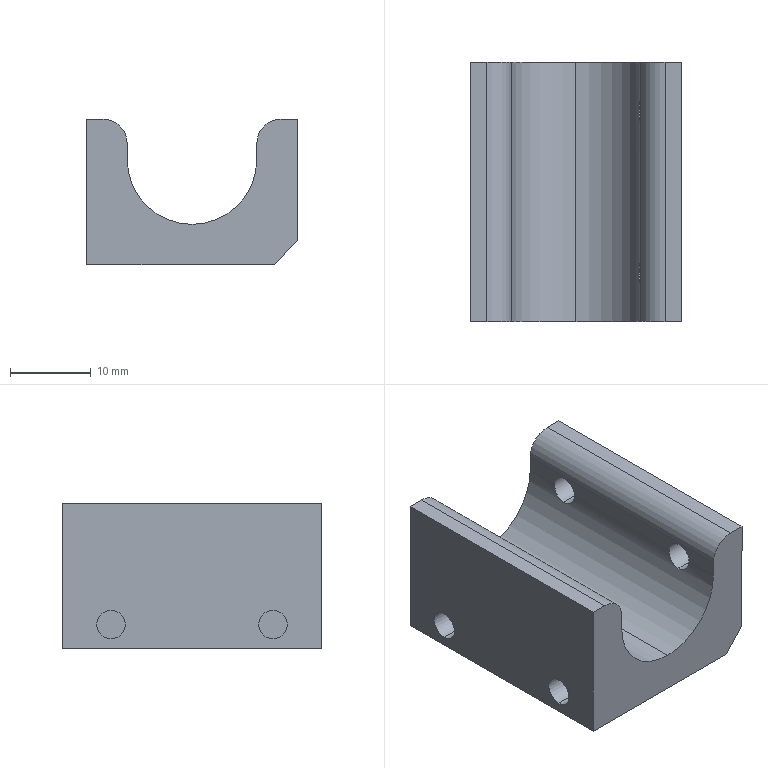Part | SolidWorks | features ICE 3, Extrusion 1 | 1 solid | 24 faces | box 26 x 32 x 18 mm | volume 8652 mm3 | cylinder 12 | plane 12 | commonest cylinder face diameters 3.5 x8 6 x2 16 x2
STEP:
#1=CARTESIAN_POINT('',(-3.,6.,-1.75));
#2=VERTEX_POINT('',#1);
#3=CARTESIAN_POINT('',(-3.,6.,1.75));
#4=VERTEX_POINT('',#3);
#5=CARTESIAN_POINT('',(-3.,6.,0.));
#6=DIRECTION('',(-1.,0.,0.));
#7=DIRECTION('',(0.,0.,1.));
#8=AXIS2_PLACEMENT_3D('',#5,#6,#7);
#9=CIRCLE('',#8,1.75);
#10=EDGE_CURVE('',#2,#4,#9,.T.);
#11=ORIENTED_EDGE('',*,*,#10,.F.);
#12=CARTESIAN_POINT('',(-13.,6.,-1.75));
#13=VERTEX_POINT('',#12);
#14=CARTESIAN_POINT('',(-3.,6.,-1.75));
#15=DIRECTION('',(-1.,0.,0.));
#16=VECTOR('',#15,1000.);
#17=LINE('',#14,#16);
#18=EDGE_CURVE('',#2,#13,#17,.T.);
#19=ORIENTED_EDGE('',*,*,#18,.T.);
#20=CARTESIAN_POINT('',(-13.,6.,1.75));
#21=VERTEX_POINT('',#20);
#22=CARTESIAN_POINT('',(-13.,6.,0.));
#23=DIRECTION('',(-1.,0.,0.));
#24=DIRECTION('',(0.,0.,1.));
#25=AXIS2_PLACEMENT_3D('',#22,#23,#24);
#26=CIRCLE('',#25,1.75);
#27=EDGE_CURVE('',#13,#21,#26,.T.);
#28=ORIENTED_EDGE('',*,*,#27,.T.);
#29=CARTESIAN_POINT('',(-3.,6.,1.75));
#30=DIRECTION('',(-1.,0.,0.));
#31=VECTOR('',#30,1000.);
#32=LINE('',#29,#31);
#33=EDGE_CURVE('',#4,#21,#32,.T.);
#34=ORIENTED_EDGE('',*,*,#33,.F.);
#35=EDGE_LOOP('',(#11,#19,#28,#34));
#36=FACE_OUTER_BOUND('',#35,.T.);
#37=CARTESIAN_POINT('',(-3.,6.,0.));
#38=DIRECTION('',(-1.,0.,0.));
#39=DIRECTION('',(0.,0.,1.));
#40=AXIS2_PLACEMENT_3D('',#37,#38,#39);
#41=CYLINDRICAL_SURFACE('',#40,1.75);
#42=ADVANCED_FACE('',(#36),#41,.F.);
#43=CARTESIAN_POINT('',(-3.,26.,-1.75));
#44=VERTEX_POINT('',#43);
#45=CARTESIAN_POINT('',(-3.,26.,1.75));
#46=VERTEX_POINT('',#45);
#47=CARTESIAN_POINT('',(-3.,26.,0.));
#48=DIRECTION('',(-1.,0.,0.));
#49=DIRECTION('',(0.,0.,1.));
#50=AXIS2_PLACEMENT_3D('',#47,#48,#49);
#51=CIRCLE('',#50,1.75);
#52=EDGE_CURVE('',#44,#46,#51,.T.);
#53=ORIENTED_EDGE('',*,*,#52,.F.);
#54=CARTESIAN_POINT('',(-13.,26.,-1.75));
#55=VERTEX_POINT('',#54);
#56=CARTESIAN_POINT('',(-3.,26.,-1.75));
#57=DIRECTION('',(-1.,0.,0.));
#58=VECTOR('',#57,1000.);
#59=LINE('',#56,#58);
#60=EDGE_CURVE('',#44,#55,#59,.T.);
#61=ORIENTED_EDGE('',*,*,#60,.T.);
#62=CARTESIAN_POINT('',(-13.,26.,1.75));
#63=VERTEX_POINT('',#62);
#64=CARTESIAN_POINT('',(-13.,26.,0.));
#65=DIRECTION('',(-1.,0.,0.));
#66=DIRECTION('',(0.,0.,1.));
#67=AXIS2_PLACEMENT_3D('',#64,#65,#66);
#68=CIRCLE('',#67,1.75);
#69=EDGE_CURVE('',#55,#63,#68,.T.);
#70=ORIENTED_EDGE('',*,*,#69,.T.);
#71=CARTESIAN_POINT('',(-3.,26.,1.75));
#72=DIRECTION('',(-1.,0.,0.));
#73=VECTOR('',#72,1000.);
#74=LINE('',#71,#73);
#75=EDGE_CURVE('',#46,#63,#74,.T.);
#76=ORIENTED_EDGE('',*,*,#75,.F.);
#77=EDGE_LOOP('',(#53,#61,#70,#76));
#78=FACE_OUTER_BOUND('',#77,.T.);
#79=CARTESIAN_POINT('',(-3.,26.,0.));
#80=DIRECTION('',(-1.,0.,0.));
#81=DIRECTION('',(0.,0.,1.));
#82=AXIS2_PLACEMENT_3D('',#79,#80,#81);
#83=CYLINDRICAL_SURFACE('',#82,1.75);
#84=ADVANCED_FACE('',(#78),#83,.F.);
#85=CARTESIAN_POINT('',(8.,26.,11.75));
#86=VERTEX_POINT('',#85);
#87=CARTESIAN_POINT('',(8.,24.25,10.));
#88=VERTEX_POINT('',#87);
#89=CARTESIAN_POINT('',(8.,26.,10.));
#90=DIRECTION('',(1.,0.,0.));
#91=DIRECTION('',(0.,0.,-1.));
#92=AXIS2_PLACEMENT_3D('',#89,#90,#91);
#93=CIRCLE('',#92,1.75);
#94=EDGE_CURVE('',#86,#88,#93,.T.);
#95=ORIENTED_EDGE('',*,*,#94,.F.);
#96=CARTESIAN_POINT('',(13.,26.,11.75));
#97=VERTEX_POINT('',#96);
#98=CARTESIAN_POINT('',(3.,26.,11.75));
#99=DIRECTION('',(1.,0.,0.));
#100=VECTOR('',#99,1000.);
#101=LINE('',#98,#100);
#102=EDGE_CURVE('',#86,#97,#101,.T.);
#103=ORIENTED_EDGE('',*,*,#102,.T.);
#104=CARTESIAN_POINT('',(13.,26.,8.25));
#105=VERTEX_POINT('',#104);
#106=CARTESIAN_POINT('',(13.,26.,10.));
#107=DIRECTION('',(1.,0.,0.));
#108=DIRECTION('',(0.,0.,-1.));
#109=AXIS2_PLACEMENT_3D('',#106,#107,#108);
#110=CIRCLE('',#109,1.75);
#111=EDGE_CURVE('',#97,#105,#110,.T.);
#112=ORIENTED_EDGE('',*,*,#111,.T.);
#113=CARTESIAN_POINT('',(7.806,26.,8.25));
#114=VERTEX_POINT('',#113);
#115=CARTESIAN_POINT('',(3.,26.,8.25));
#116=DIRECTION('',(1.,0.,0.));
#117=VECTOR('',#116,1000.);
#118=LINE('',#115,#117);
#119=EDGE_CURVE('',#114,#105,#118,.T.);
#120=ORIENTED_EDGE('',*,*,#119,.F.);
#121=CARTESIAN_POINT('',(8.,24.25,10.));
#122=CARTESIAN_POINT('',(8.,24.25,9.884));
#123=CARTESIAN_POINT('',(7.997,24.261,9.77));
#124=CARTESIAN_POINT('',(7.988,24.306,9.546));
#125=CARTESIAN_POINT('',(7.981,24.34,9.434));
#126=CARTESIAN_POINT('',(7.963,24.428,9.223));
#127=CARTESIAN_POINT('',(7.952,24.482,9.122));
#128=CARTESIAN_POINT('',(7.929,24.609,8.932));
#129=CARTESIAN_POINT('',(7.916,24.683,8.842));
#130=CARTESIAN_POINT('',(7.878,24.924,8.601));
#131=CARTESIAN_POINT('',(7.853,25.119,8.471));
#132=CARTESIAN_POINT('',(7.817,25.54,8.296));
#133=CARTESIAN_POINT('',(7.806,25.771,8.25));
#134=CARTESIAN_POINT('',(7.806,26.,8.25));
#135=B_SPLINE_CURVE_WITH_KNOTS('',3,(#121,#122,#123,#124,#125,#126,#127,#128,#129,#130,#131,#132,#133,#134),.UNSPECIFIED.,.F.,.F.,(4,2,2,2,2,2,4),(0.,0.0003431,0.0006862,0.001029,0.001372,0.002058,0.002745),.UNSPECIFIED.);
#136=EDGE_CURVE('',#88,#114,#135,.T.);
#137=ORIENTED_EDGE('',*,*,#136,.F.);
#138=EDGE_LOOP('',(#95,#103,#112,#120,#137));
#139=FACE_OUTER_BOUND('',#138,.T.);
#140=CARTESIAN_POINT('',(3.,26.,10.));
#141=DIRECTION('',(1.,0.,0.));
#142=DIRECTION('',(0.,0.,-1.));
#143=AXIS2_PLACEMENT_3D('',#140,#141,#142);
#144=CYLINDRICAL_SURFACE('',#143,1.75);
#145=ADVANCED_FACE('',(#139),#144,.F.);
#146=CARTESIAN_POINT('',(8.,6.,11.75));
#147=VERTEX_POINT('',#146);
#148=CARTESIAN_POINT('',(8.,4.25,10.));
#149=VERTEX_POINT('',#148);
#150=CARTESIAN_POINT('',(8.,6.,10.));
#151=DIRECTION('',(1.,0.,0.));
#152=DIRECTION('',(0.,0.,-1.));
#153=AXIS2_PLACEMENT_3D('',#150,#151,#152);
#154=CIRCLE('',#153,1.75);
#155=EDGE_CURVE('',#147,#149,#154,.T.);
#156=ORIENTED_EDGE('',*,*,#155,.F.);
#157=CARTESIAN_POINT('',(13.,6.,11.75));
#158=VERTEX_POINT('',#157);
#159=CARTESIAN_POINT('',(3.,6.,11.75));
#160=DIRECTION('',(1.,0.,0.));
#161=VECTOR('',#160,1000.);
#162=LINE('',#159,#161);
#163=EDGE_CURVE('',#147,#158,#162,.T.);
#164=ORIENTED_EDGE('',*,*,#163,.T.);
#165=CARTESIAN_POINT('',(13.,6.,8.25));
#166=VERTEX_POINT('',#165);
#167=CARTESIAN_POINT('',(13.,6.,10.));
#168=DIRECTION('',(1.,0.,0.));
#169=DIRECTION('',(0.,0.,-1.));
#170=AXIS2_PLACEMENT_3D('',#167,#168,#169);
#171=CIRCLE('',#170,1.75);
#172=EDGE_CURVE('',#158,#166,#171,.T.);
#173=ORIENTED_EDGE('',*,*,#172,.T.);
#174=CARTESIAN_POINT('',(7.806,6.,8.25));
#175=VERTEX_POINT('',#174);
#176=CARTESIAN_POINT('',(3.,6.,8.25));
#177=DIRECTION('',(1.,0.,0.));
#178=VECTOR('',#177,1000.);
#179=LINE('',#176,#178);
#180=EDGE_CURVE('',#175,#166,#179,.T.);
#181=ORIENTED_EDGE('',*,*,#180,.F.);
#182=CARTESIAN_POINT('',(8.,4.25,10.));
#183=CARTESIAN_POINT('',(8.,4.25,9.884));
#184=CARTESIAN_POINT('',(7.997,4.261,9.77));
#185=CARTESIAN_POINT('',(7.988,4.306,9.546));
#186=CARTESIAN_POINT('',(7.981,4.34,9.434));
#187=CARTESIAN_POINT('',(7.963,4.428,9.223));
#188=CARTESIAN_POINT('',(7.952,4.482,9.122));
#189=CARTESIAN_POINT('',(7.929,4.609,8.932));
#190=CARTESIAN_POINT('',(7.916,4.683,8.842));
#191=CARTESIAN_POINT('',(7.878,4.924,8.601));
#192=CARTESIAN_POINT('',(7.853,5.119,8.471));
#193=CARTESIAN_POINT('',(7.817,5.54,8.296));
#194=CARTESIAN_POINT('',(7.806,5.771,8.25));
#195=CARTESIAN_POINT('',(7.806,6.,8.25));
#196=B_SPLINE_CURVE_WITH_KNOTS('',3,(#182,#183,#184,#185,#186,#187,#188,#189,#190,#191,#192,#193,#194,#195),.UNSPECIFIED.,.F.,.F.,(4,2,2,2,2,2,4),(0.,0.0003431,0.0006862,0.001029,0.001372,0.002058,0.002745),.UNSPECIFIED.);
#197=EDGE_CURVE('',#149,#175,#196,.T.);
#198=ORIENTED_EDGE('',*,*,#197,.F.);
#199=EDGE_LOOP('',(#156,#164,#173,#181,#198));
#200=FACE_OUTER_BOUND('',#199,.T.);
#201=CARTESIAN_POINT('',(3.,6.,10.));
#202=DIRECTION('',(1.,0.,0.));
#203=DIRECTION('',(0.,0.,-1.));
#204=AXIS2_PLACEMENT_3D('',#201,#202,#203);
#205=CYLINDRICAL_SURFACE('',#204,1.75);
#206=ADVANCED_FACE('',(#200),#205,.F.);
#207=CARTESIAN_POINT('',(0.,32.,2.));
#208=VERTEX_POINT('',#207);
#209=CARTESIAN_POINT('',(8.,32.,10.));
#210=VERTEX_POINT('',#209);
#211=CARTESIAN_POINT('',(0.,32.,10.));
#212=DIRECTION('',(0.,-1.,0.));
#213=DIRECTION('',(0.,0.,1.));
#214=AXIS2_PLACEMENT_3D('',#211,#212,#213);
#215=CIRCLE('',#214,8.);
#216=EDGE_CURVE('',#208,#210,#215,.T.);
#217=ORIENTED_EDGE('',*,*,#216,.F.);
#218=CARTESIAN_POINT('',(0.,0.,2.));
#219=VERTEX_POINT('',#218);
#220=CARTESIAN_POINT('',(0.,32.,2.));
#221=DIRECTION('',(0.,-1.,0.));
#222=VECTOR('',#221,1000.);
#223=LINE('',#220,#222);
#224=EDGE_CURVE('',#208,#219,#223,.T.);
#225=ORIENTED_EDGE('',*,*,#224,.T.);
#226=CARTESIAN_POINT('',(8.,0.,10.));
#227=VERTEX_POINT('',#226);
#228=CARTESIAN_POINT('',(0.,0.,10.));
#229=DIRECTION('',(0.,-1.,0.));
#230=DIRECTION('',(0.,0.,1.));
#231=AXIS2_PLACEMENT_3D('',#228,#229,#230);
#232=CIRCLE('',#231,8.);
#233=EDGE_CURVE('',#219,#227,#232,.T.);
#234=ORIENTED_EDGE('',*,*,#233,.T.);
#235=CARTESIAN_POINT('',(8.,32.,10.));
#236=DIRECTION('',(0.,-1.,0.));
#237=VECTOR('',#236,1000.);
#238=LINE('',#235,#237);
#239=EDGE_CURVE('',#149,#227,#238,.T.);
#240=ORIENTED_EDGE('',*,*,#239,.F.);
#241=ORIENTED_EDGE('',*,*,#197,.T.);
#242=CARTESIAN_POINT('',(8.,7.75,10.));
#243=VERTEX_POINT('',#242);
#244=CARTESIAN_POINT('',(7.806,6.,8.25));
#245=CARTESIAN_POINT('',(7.806,6.114,8.25));
#246=CARTESIAN_POINT('',(7.809,6.231,8.262));
#247=CARTESIAN_POINT('',(7.819,6.455,8.306));
#248=CARTESIAN_POINT('',(7.826,6.564,8.34));
#249=CARTESIAN_POINT('',(7.853,6.883,8.472));
#250=CARTESIAN_POINT('',(7.878,7.075,8.6));
#251=CARTESIAN_POINT('',(7.916,7.318,8.844));
#252=CARTESIAN_POINT('',(7.929,7.391,8.931));
#253=CARTESIAN_POINT('',(7.952,7.517,9.121));
#254=CARTESIAN_POINT('',(7.963,7.572,9.223));
#255=CARTESIAN_POINT('',(7.99,7.704,9.54));
#256=CARTESIAN_POINT('',(8.,7.75,9.768));
#257=CARTESIAN_POINT('',(8.,7.75,10.));
#258=B_SPLINE_CURVE_WITH_KNOTS('',3,(#244,#245,#246,#247,#248,#249,#250,#251,#252,#253,#254,#255,#256,#257),.UNSPECIFIED.,.F.,.F.,(4,2,2,2,2,2,4),(0.002745,0.003087,0.00343,0.004116,0.004458,0.004801,0.005486),.UNSPECIFIED.);
#259=EDGE_CURVE('',#175,#243,#258,.T.);
#260=ORIENTED_EDGE('',*,*,#259,.T.);
#261=CARTESIAN_POINT('',(8.,32.,10.));
#262=DIRECTION('',(0.,-1.,0.));
#263=VECTOR('',#262,1000.);
#264=LINE('',#261,#263);
#265=EDGE_CURVE('',#88,#243,#264,.T.);
#266=ORIENTED_EDGE('',*,*,#265,.F.);
#267=ORIENTED_EDGE('',*,*,#136,.T.);
#268=CARTESIAN_POINT('',(8.,27.75,10.));
#269=VERTEX_POINT('',#268);
#270=CARTESIAN_POINT('',(7.806,26.,8.25));
#271=CARTESIAN_POINT('',(7.806,26.114,8.25));
#272=CARTESIAN_POINT('',(7.809,26.231,8.262));
#273=CARTESIAN_POINT('',(7.819,26.455,8.306));
#274=CARTESIAN_POINT('',(7.826,26.564,8.34));
#275=CARTESIAN_POINT('',(7.853,26.883,8.472));
#276=CARTESIAN_POINT('',(7.878,27.075,8.6));
#277=CARTESIAN_POINT('',(7.916,27.318,8.844));
#278=CARTESIAN_POINT('',(7.929,27.391,8.931));
#279=CARTESIAN_POINT('',(7.952,27.517,9.121));
#280=CARTESIAN_POINT('',(7.963,27.572,9.223));
#281=CARTESIAN_POINT('',(7.99,27.704,9.54));
#282=CARTESIAN_POINT('',(8.,27.75,9.768));
#283=CARTESIAN_POINT('',(8.,27.75,10.));
#284=B_SPLINE_CURVE_WITH_KNOTS('',3,(#270,#271,#272,#273,#274,#275,#276,#277,#278,#279,#280,#281,#282,#283),.UNSPECIFIED.,.F.,.F.,(4,2,2,2,2,2,4),(0.002745,0.003087,0.00343,0.004116,0.004458,0.004801,0.005486),.UNSPECIFIED.);
#285=EDGE_CURVE('',#114,#269,#284,.T.);
#286=ORIENTED_EDGE('',*,*,#285,.T.);
#287=CARTESIAN_POINT('',(8.,32.,10.));
#288=DIRECTION('',(0.,-1.,0.));
#289=VECTOR('',#288,1000.);
#290=LINE('',#287,#289);
#291=EDGE_CURVE('',#210,#269,#290,.T.);
#292=ORIENTED_EDGE('',*,*,#291,.F.);
#293=EDGE_LOOP('',(#217,#225,#234,#240,#241,#260,#266,#267,#286,#292));
#294=FACE_OUTER_BOUND('',#293,.T.);
#295=CARTESIAN_POINT('',(0.,32.,10.));
#296=DIRECTION('',(0.,-1.,0.));
#297=DIRECTION('',(0.,0.,-1.));
#298=AXIS2_PLACEMENT_3D('',#295,#296,#297);
#299=CYLINDRICAL_SURFACE('',#298,8.);
#300=ADVANCED_FACE('',(#294),#299,.F.);
#301=CARTESIAN_POINT('',(8.,0.,12.));
#302=VERTEX_POINT('',#301);
#303=CARTESIAN_POINT('',(11.,0.,15.));
#304=VERTEX_POINT('',#303);
#305=CARTESIAN_POINT('',(11.,0.,12.));
#306=DIRECTION('',(0.,1.,0.));
#307=DIRECTION('',(0.,0.,1.));
#308=AXIS2_PLACEMENT_3D('',#305,#306,#307);
#309=CIRCLE('',#308,3.);
#310=EDGE_CURVE('',#302,#304,#309,.T.);
#311=ORIENTED_EDGE('',*,*,#310,.T.);
#312=CARTESIAN_POINT('',(11.,32.,15.));
#313=VERTEX_POINT('',#312);
#314=CARTESIAN_POINT('',(11.,32.,15.));
#315=DIRECTION('',(0.,-1.,0.));
#316=VECTOR('',#315,1000.);
#317=LINE('',#314,#316);
#318=EDGE_CURVE('',#313,#304,#317,.T.);
#319=ORIENTED_EDGE('',*,*,#318,.F.);
#320=CARTESIAN_POINT('',(8.,32.,12.));
#321=VERTEX_POINT('',#320);
#322=CARTESIAN_POINT('',(11.,32.,12.));
#323=DIRECTION('',(0.,1.,0.));
#324=DIRECTION('',(0.,0.,1.));
#325=AXIS2_PLACEMENT_3D('',#322,#323,#324);
#326=CIRCLE('',#325,3.);
#327=EDGE_CURVE('',#321,#313,#326,.T.);
#328=ORIENTED_EDGE('',*,*,#327,.F.);
#329=CARTESIAN_POINT('',(8.,32.,12.));
#330=DIRECTION('',(0.,-1.,0.));
#331=VECTOR('',#330,1000.);
#332=LINE('',#329,#331);
#333=EDGE_CURVE('',#321,#302,#332,.T.);
#334=ORIENTED_EDGE('',*,*,#333,.T.);
#335=EDGE_LOOP('',(#311,#319,#328,#334));
#336=FACE_OUTER_BOUND('',#335,.T.);
#337=CARTESIAN_POINT('',(11.,32.,12.));
#338=DIRECTION('',(0.,-1.,0.));
#339=DIRECTION('',(0.,0.,-1.));
#340=AXIS2_PLACEMENT_3D('',#337,#338,#339);
#341=CYLINDRICAL_SURFACE('',#340,3.);
#342=ADVANCED_FACE('',(#336),#341,.T.);
#343=CARTESIAN_POINT('',(13.,0.,15.));
#344=VERTEX_POINT('',#343);
#345=CARTESIAN_POINT('',(11.,0.,15.));
#346=DIRECTION('',(1.,0.,0.));
#347=VECTOR('',#346,1000.);
#348=LINE('',#345,#347);
#349=EDGE_CURVE('',#304,#344,#348,.T.);
#350=ORIENTED_EDGE('',*,*,#349,.T.);
#351=CARTESIAN_POINT('',(13.,32.,15.));
#352=VERTEX_POINT('',#351);
#353=CARTESIAN_POINT('',(13.,32.,15.));
#354=DIRECTION('',(0.,-1.,0.));
#355=VECTOR('',#354,1000.);
#356=LINE('',#353,#355);
#357=EDGE_CURVE('',#352,#344,#356,.T.);
#358=ORIENTED_EDGE('',*,*,#357,.F.);
#359=CARTESIAN_POINT('',(11.,32.,15.));
#360=DIRECTION('',(1.,0.,0.));
#361=VECTOR('',#360,1000.);
#362=LINE('',#359,#361);
#363=EDGE_CURVE('',#313,#352,#362,.T.);
#364=ORIENTED_EDGE('',*,*,#363,.F.);
#365=ORIENTED_EDGE('',*,*,#318,.T.);
#366=EDGE_LOOP('',(#350,#358,#364,#365));
#367=FACE_OUTER_BOUND('',#366,.T.);
#368=CARTESIAN_POINT('',(11.,32.,15.));
#369=DIRECTION('',(0.,0.,-1.));
#370=DIRECTION('',(-1.,0.,0.));
#371=AXIS2_PLACEMENT_3D('',#368,#369,#370);
#372=PLANE('',#371);
#373=ADVANCED_FACE('',(#367),#372,.F.);
#374=CARTESIAN_POINT('',(13.,26.,10.));
#375=DIRECTION('',(1.,0.,0.));
#376=DIRECTION('',(0.,0.,-1.));
#377=AXIS2_PLACEMENT_3D('',#374,#375,#376);
#378=CIRCLE('',#377,1.75);
#379=EDGE_CURVE('',#105,#97,#378,.T.);
#380=ORIENTED_EDGE('',*,*,#379,.F.);
#381=ORIENTED_EDGE('',*,*,#111,.F.);
#382=EDGE_LOOP('',(#380,#381));
#383=FACE_BOUND('',#382,.T.);
#384=CARTESIAN_POINT('',(13.,6.,10.));
#385=DIRECTION('',(1.,0.,0.));
#386=DIRECTION('',(0.,0.,-1.));
#387=AXIS2_PLACEMENT_3D('',#384,#385,#386);
#388=CIRCLE('',#387,1.75);
#389=EDGE_CURVE('',#166,#158,#388,.T.);
#390=ORIENTED_EDGE('',*,*,#389,.F.);
#391=ORIENTED_EDGE('',*,*,#172,.F.);
#392=EDGE_LOOP('',(#390,#391));
#393=FACE_BOUND('',#392,.T.);
#394=CARTESIAN_POINT('',(13.,0.,0.));
#395=VERTEX_POINT('',#394);
#396=CARTESIAN_POINT('',(13.,0.,15.));
#397=DIRECTION('',(0.,0.,-1.));
#398=VECTOR('',#397,1000.);
#399=LINE('',#396,#398);
#400=EDGE_CURVE('',#344,#395,#399,.T.);
#401=ORIENTED_EDGE('',*,*,#400,.T.);
#402=CARTESIAN_POINT('',(13.,32.,0.));
#403=VERTEX_POINT('',#402);
#404=CARTESIAN_POINT('',(13.,32.,0.));
#405=DIRECTION('',(0.,-1.,0.));
#406=VECTOR('',#405,1000.);
#407=LINE('',#404,#406);
#408=EDGE_CURVE('',#403,#395,#407,.T.);
#409=ORIENTED_EDGE('',*,*,#408,.F.);
#410=CARTESIAN_POINT('',(13.,32.,15.));
#411=DIRECTION('',(0.,0.,-1.));
#412=VECTOR('',#411,1000.);
#413=LINE('',#410,#412);
#414=EDGE_CURVE('',#352,#403,#413,.T.);
#415=ORIENTED_EDGE('',*,*,#414,.F.);
#416=ORIENTED_EDGE('',*,*,#357,.T.);
#417=EDGE_LOOP('',(#401,#409,#415,#416));
#418=FACE_OUTER_BOUND('',#417,.T.);
#419=CARTESIAN_POINT('',(13.,32.,15.));
#420=DIRECTION('',(-1.,0.,0.));
#421=DIRECTION('',(0.,0.,1.));
#422=AXIS2_PLACEMENT_3D('',#419,#420,#421);
#423=PLANE('',#422);
#424=ADVANCED_FACE('',(#383,#393,#418),#423,.F.);
#425=CARTESIAN_POINT('',(10.2,0.,-3.));
#426=VERTEX_POINT('',#425);
#427=CARTESIAN_POINT('',(13.,0.,0.));
#428=DIRECTION('',(-0.6823,0.,-0.7311));
#429=VECTOR('',#428,1000.);
#430=LINE('',#427,#429);
#431=EDGE_CURVE('',#395,#426,#430,.T.);
#432=ORIENTED_EDGE('',*,*,#431,.T.);
#433=CARTESIAN_POINT('',(10.2,32.,-3.));
#434=VERTEX_POINT('',#433);
#435=CARTESIAN_POINT('',(10.2,32.,-3.));
#436=DIRECTION('',(0.,1.,0.));
#437=VECTOR('',#436,1000.);
#438=LINE('',#435,#437);
#439=EDGE_CURVE('',#426,#434,#438,.T.);
#440=ORIENTED_EDGE('',*,*,#439,.T.);
#441=CARTESIAN_POINT('',(13.,32.,0.));
#442=DIRECTION('',(-0.6823,0.,-0.7311));
#443=VECTOR('',#442,1000.);
#444=LINE('',#441,#443);
#445=EDGE_CURVE('',#403,#434,#444,.T.);
#446=ORIENTED_EDGE('',*,*,#445,.F.);
#447=ORIENTED_EDGE('',*,*,#408,.T.);
#448=EDGE_LOOP('',(#432,#440,#446,#447));
#449=FACE_OUTER_BOUND('',#448,.T.);
#450=CARTESIAN_POINT('',(13.,32.,0.));
#451=DIRECTION('',(-0.7311,0.,0.6823));
#452=DIRECTION('',(0.6823,0.,0.7311));
#453=AXIS2_PLACEMENT_3D('',#450,#451,#452);
#454=PLANE('',#453);
#455=ADVANCED_FACE('',(#449),#454,.F.);
#456=CARTESIAN_POINT('',(-13.,6.,0.));
#457=DIRECTION('',(-1.,0.,0.));
#458=DIRECTION('',(0.,0.,1.));
#459=AXIS2_PLACEMENT_3D('',#456,#457,#458);
#460=CIRCLE('',#459,1.75);
#461=EDGE_CURVE('',#21,#13,#460,.T.);
#462=ORIENTED_EDGE('',*,*,#461,.F.);
#463=ORIENTED_EDGE('',*,*,#27,.F.);
#464=EDGE_LOOP('',(#462,#463));
#465=FACE_BOUND('',#464,.T.);
#466=CARTESIAN_POINT('',(-13.,26.,0.));
#467=DIRECTION('',(-1.,0.,0.));
#468=DIRECTION('',(0.,0.,1.));
#469=AXIS2_PLACEMENT_3D('',#466,#467,#468);
#470=CIRCLE('',#469,1.75);
#471=EDGE_CURVE('',#63,#55,#470,.T.);
#472=ORIENTED_EDGE('',*,*,#471,.F.);
#473=ORIENTED_EDGE('',*,*,#69,.F.);
#474=EDGE_LOOP('',(#472,#473));
#475=FACE_BOUND('',#474,.T.);
#476=CARTESIAN_POINT('',(-13.,32.,-3.));
#477=VERTEX_POINT('',#476);
#478=CARTESIAN_POINT('',(-13.,32.,15.));
#479=VERTEX_POINT('',#478);
#480=CARTESIAN_POINT('',(-13.,32.,15.));
#481=DIRECTION('',(0.,0.,1.));
#482=VECTOR('',#481,1000.);
#483=LINE('',#480,#482);
#484=EDGE_CURVE('',#477,#479,#483,.T.);
#485=ORIENTED_EDGE('',*,*,#484,.F.);
#486=CARTESIAN_POINT('',(-13.,0.,-3.));
#487=VERTEX_POINT('',#486);
#488=CARTESIAN_POINT('',(-13.,32.,-3.));
#489=DIRECTION('',(0.,-1.,0.));
#490=VECTOR('',#489,1000.);
#491=LINE('',#488,#490);
#492=EDGE_CURVE('',#477,#487,#491,.T.);
#493=ORIENTED_EDGE('',*,*,#492,.T.);
#494=CARTESIAN_POINT('',(-13.,0.,15.));
#495=VERTEX_POINT('',#494);
#496=CARTESIAN_POINT('',(-13.,0.,15.));
#497=DIRECTION('',(0.,0.,1.));
#498=VECTOR('',#497,1000.);
#499=LINE('',#496,#498);
#500=EDGE_CURVE('',#487,#495,#499,.T.);
#501=ORIENTED_EDGE('',*,*,#500,.T.);
#502=CARTESIAN_POINT('',(-13.,32.,15.));
#503=DIRECTION('',(0.,-1.,0.));
#504=VECTOR('',#503,1000.);
#505=LINE('',#502,#504);
#506=EDGE_CURVE('',#479,#495,#505,.T.);
#507=ORIENTED_EDGE('',*,*,#506,.F.);
#508=EDGE_LOOP('',(#485,#493,#501,#507));
#509=FACE_OUTER_BOUND('',#508,.T.);
#510=CARTESIAN_POINT('',(-13.,32.,15.));
#511=DIRECTION('',(1.,0.,0.));
#512=DIRECTION('',(0.,0.,-1.));
#513=AXIS2_PLACEMENT_3D('',#510,#511,#512);
#514=PLANE('',#513);
#515=ADVANCED_FACE('',(#465,#475,#509),#514,.F.);
#516=CARTESIAN_POINT('',(-11.,0.,15.));
#517=VERTEX_POINT('',#516);
#518=CARTESIAN_POINT('',(-13.,0.,15.));
#519=DIRECTION('',(1.,0.,0.));
#520=VECTOR('',#519,1000.);
#521=LINE('',#518,#520);
#522=EDGE_CURVE('',#495,#517,#521,.T.);
#523=ORIENTED_EDGE('',*,*,#522,.T.);
#524=CARTESIAN_POINT('',(-11.,32.,15.));
#525=VERTEX_POINT('',#524);
#526=CARTESIAN_POINT('',(-11.,32.,15.));
#527=DIRECTION('',(0.,-1.,0.));
#528=VECTOR('',#527,1000.);
#529=LINE('',#526,#528);
#530=EDGE_CURVE('',#525,#517,#529,.T.);
#531=ORIENTED_EDGE('',*,*,#530,.F.);
#532=CARTESIAN_POINT('',(-13.,32.,15.));
#533=DIRECTION('',(1.,0.,0.));
#534=VECTOR('',#533,1000.);
#535=LINE('',#532,#534);
#536=EDGE_CURVE('',#479,#525,#535,.T.);
#537=ORIENTED_EDGE('',*,*,#536,.F.);
#538=ORIENTED_EDGE('',*,*,#506,.T.);
#539=EDGE_LOOP('',(#523,#531,#537,#538));
#540=FACE_OUTER_BOUND('',#539,.T.);
#541=CARTESIAN_POINT('',(-13.,32.,15.));
#542=DIRECTION('',(0.,0.,-1.));
#543=DIRECTION('',(-1.,0.,0.));
#544=AXIS2_PLACEMENT_3D('',#541,#542,#543);
#545=PLANE('',#544);
#546=ADVANCED_FACE('',(#540),#545,.F.);
#547=CARTESIAN_POINT('',(-8.,0.,12.));
#548=VERTEX_POINT('',#547);
#549=CARTESIAN_POINT('',(-11.,0.,12.));
#550=DIRECTION('',(0.,1.,0.));
#551=DIRECTION('',(0.,0.,-1.));
#552=AXIS2_PLACEMENT_3D('',#549,#550,#551);
#553=CIRCLE('',#552,3.);
#554=EDGE_CURVE('',#517,#548,#553,.T.);
#555=ORIENTED_EDGE('',*,*,#554,.T.);
#556=CARTESIAN_POINT('',(-8.,32.,12.));
#557=VERTEX_POINT('',#556);
#558=CARTESIAN_POINT('',(-8.,32.,12.));
#559=DIRECTION('',(0.,-1.,0.));
#560=VECTOR('',#559,1000.);
#561=LINE('',#558,#560);
#562=EDGE_CURVE('',#557,#548,#561,.T.);
#563=ORIENTED_EDGE('',*,*,#562,.F.);
#564=CARTESIAN_POINT('',(-11.,32.,12.));
#565=DIRECTION('',(0.,1.,0.));
#566=DIRECTION('',(0.,0.,-1.));
#567=AXIS2_PLACEMENT_3D('',#564,#565,#566);
#568=CIRCLE('',#567,3.);
#569=EDGE_CURVE('',#525,#557,#568,.T.);
#570=ORIENTED_EDGE('',*,*,#569,.F.);
#571=ORIENTED_EDGE('',*,*,#530,.T.);
#572=EDGE_LOOP('',(#555,#563,#570,#571));
#573=FACE_OUTER_BOUND('',#572,.T.);
#574=CARTESIAN_POINT('',(-11.,32.,12.));
#575=DIRECTION('',(0.,-1.,0.));
#576=DIRECTION('',(0.,0.,-1.));
#577=AXIS2_PLACEMENT_3D('',#574,#575,#576);
#578=CYLINDRICAL_SURFACE('',#577,3.);
#579=ADVANCED_FACE('',(#573),#578,.T.);
#580=CARTESIAN_POINT('',(-8.,0.,10.));
#581=VERTEX_POINT('',#580);
#582=CARTESIAN_POINT('',(-8.,0.,10.));
#583=DIRECTION('',(0.,0.,-1.));
#584=VECTOR('',#583,1000.);
#585=LINE('',#582,#584);
#586=EDGE_CURVE('',#548,#581,#585,.T.);
#587=ORIENTED_EDGE('',*,*,#586,.T.);
#588=CARTESIAN_POINT('',(-8.,32.,10.));
#589=VERTEX_POINT('',#588);
#590=CARTESIAN_POINT('',(-8.,32.,10.));
#591=DIRECTION('',(0.,-1.,0.));
#592=VECTOR('',#591,1000.);
#593=LINE('',#590,#592);
#594=EDGE_CURVE('',#589,#581,#593,.T.);
#595=ORIENTED_EDGE('',*,*,#594,.F.);
#596=CARTESIAN_POINT('',(-8.,32.,10.));
#597=DIRECTION('',(0.,0.,-1.));
#598=VECTOR('',#597,1000.);
#599=LINE('',#596,#598);
#600=EDGE_CURVE('',#557,#589,#599,.T.);
#601=ORIENTED_EDGE('',*,*,#600,.F.);
#602=ORIENTED_EDGE('',*,*,#562,.T.);
#603=EDGE_LOOP('',(#587,#595,#601,#602));
#604=FACE_OUTER_BOUND('',#603,.T.);
#605=CARTESIAN_POINT('',(-8.,32.,10.));
#606=DIRECTION('',(-1.,0.,0.));
#607=DIRECTION('',(0.,0.,1.));
#608=AXIS2_PLACEMENT_3D('',#605,#606,#607);
#609=PLANE('',#608);
#610=ADVANCED_FACE('',(#604),#609,.F.);
#611=ORIENTED_EDGE('',*,*,#224,.F.);
#612=CARTESIAN_POINT('',(0.,32.,10.));
#613=DIRECTION('',(0.,-1.,0.));
#614=DIRECTION('',(0.,0.,1.));
#615=AXIS2_PLACEMENT_3D('',#612,#613,#614);
#616=CIRCLE('',#615,8.);
#617=EDGE_CURVE('',#589,#208,#616,.T.);
#618=ORIENTED_EDGE('',*,*,#617,.F.);
#619=ORIENTED_EDGE('',*,*,#594,.T.);
#620=CARTESIAN_POINT('',(0.,0.,10.));
#621=DIRECTION('',(0.,-1.,0.));
#622=DIRECTION('',(0.,0.,1.));
#623=AXIS2_PLACEMENT_3D('',#620,#621,#622);
#624=CIRCLE('',#623,8.);
#625=EDGE_CURVE('',#581,#219,#624,.T.);
#626=ORIENTED_EDGE('',*,*,#625,.T.);
#627=EDGE_LOOP('',(#611,#618,#619,#626));
#628=FACE_OUTER_BOUND('',#627,.T.);
#629=CARTESIAN_POINT('',(0.,32.,10.));
#630=DIRECTION('',(0.,-1.,0.));
#631=DIRECTION('',(0.,0.,-1.));
#632=AXIS2_PLACEMENT_3D('',#629,#630,#631);
#633=CYLINDRICAL_SURFACE('',#632,8.);
#634=ADVANCED_FACE('',(#628),#633,.F.);
#635=ORIENTED_EDGE('',*,*,#291,.T.);
#636=CARTESIAN_POINT('',(8.,26.,10.));
#637=DIRECTION('',(1.,0.,0.));
#638=DIRECTION('',(0.,0.,-1.));
#639=AXIS2_PLACEMENT_3D('',#636,#637,#638);
#640=CIRCLE('',#639,1.75);
#641=EDGE_CURVE('',#269,#86,#640,.T.);
#642=ORIENTED_EDGE('',*,*,#641,.T.);
#643=ORIENTED_EDGE('',*,*,#94,.T.);
#644=ORIENTED_EDGE('',*,*,#265,.T.);
#645=CARTESIAN_POINT('',(8.,6.,10.));
#646=DIRECTION('',(1.,0.,0.));
#647=DIRECTION('',(0.,0.,-1.));
#648=AXIS2_PLACEMENT_3D('',#645,#646,#647);
#649=CIRCLE('',#648,1.75);
#650=EDGE_CURVE('',#243,#147,#649,.T.);
#651=ORIENTED_EDGE('',*,*,#650,.T.);
#652=ORIENTED_EDGE('',*,*,#155,.T.);
#653=ORIENTED_EDGE('',*,*,#239,.T.);
#654=CARTESIAN_POINT('',(8.,0.,10.));
#655=DIRECTION('',(0.,0.,1.));
#656=VECTOR('',#655,1000.);
#657=LINE('',#654,#656);
#658=EDGE_CURVE('',#227,#302,#657,.T.);
#659=ORIENTED_EDGE('',*,*,#658,.T.);
#660=ORIENTED_EDGE('',*,*,#333,.F.);
#661=CARTESIAN_POINT('',(8.,32.,10.));
#662=DIRECTION('',(0.,0.,1.));
#663=VECTOR('',#662,1000.);
#664=LINE('',#661,#663);
#665=EDGE_CURVE('',#210,#321,#664,.T.);
#666=ORIENTED_EDGE('',*,*,#665,.F.);
#667=EDGE_LOOP('',(#635,#642,#643,#644,#651,#652,#653,#659,#660,#666));
#668=FACE_OUTER_BOUND('',#667,.T.);
#669=CARTESIAN_POINT('',(8.,32.,10.));
#670=DIRECTION('',(1.,0.,0.));
#671=DIRECTION('',(0.,0.,-1.));
#672=AXIS2_PLACEMENT_3D('',#669,#670,#671);
#673=PLANE('',#672);
#674=ADVANCED_FACE('',(#668),#673,.F.);
#675=CARTESIAN_POINT('',(-42.974,32.,-3.));
#676=DIRECTION('',(1.,0.,0.));
#677=VECTOR('',#676,1000.);
#678=LINE('',#675,#677);
#679=EDGE_CURVE('',#477,#434,#678,.T.);
#680=ORIENTED_EDGE('',*,*,#679,.F.);
#681=ORIENTED_EDGE('',*,*,#484,.T.);
#682=ORIENTED_EDGE('',*,*,#536,.T.);
#683=ORIENTED_EDGE('',*,*,#569,.T.);
#684=ORIENTED_EDGE('',*,*,#600,.T.);
#685=ORIENTED_EDGE('',*,*,#617,.T.);
#686=ORIENTED_EDGE('',*,*,#216,.T.);
#687=ORIENTED_EDGE('',*,*,#665,.T.);
#688=ORIENTED_EDGE('',*,*,#327,.T.);
#689=ORIENTED_EDGE('',*,*,#363,.T.);
#690=ORIENTED_EDGE('',*,*,#414,.T.);
#691=ORIENTED_EDGE('',*,*,#445,.T.);
#692=EDGE_LOOP('',(#680,#681,#682,#683,#684,#685,#686,#687,#688,#689,#690,#691));
#693=FACE_OUTER_BOUND('',#692,.T.);
#694=CARTESIAN_POINT('',(11.,32.,12.));
#695=DIRECTION('',(0.,1.,0.));
#696=DIRECTION('',(0.,0.,1.));
#697=AXIS2_PLACEMENT_3D('',#694,#695,#696);
#698=PLANE('',#697);
#699=ADVANCED_FACE('',(#693),#698,.T.);
#700=ORIENTED_EDGE('',*,*,#500,.F.);
#701=CARTESIAN_POINT('',(11.,0.,-3.));
#702=DIRECTION('',(1.,0.,0.));
#703=VECTOR('',#702,1000.);
#704=LINE('',#701,#703);
#705=EDGE_CURVE('',#487,#426,#704,.T.);
#706=ORIENTED_EDGE('',*,*,#705,.T.);
#707=ORIENTED_EDGE('',*,*,#431,.F.);
#708=ORIENTED_EDGE('',*,*,#400,.F.);
#709=ORIENTED_EDGE('',*,*,#349,.F.);
#710=ORIENTED_EDGE('',*,*,#310,.F.);
#711=ORIENTED_EDGE('',*,*,#658,.F.);
#712=ORIENTED_EDGE('',*,*,#233,.F.);
#713=ORIENTED_EDGE('',*,*,#625,.F.);
#714=ORIENTED_EDGE('',*,*,#586,.F.);
#715=ORIENTED_EDGE('',*,*,#554,.F.);
#716=ORIENTED_EDGE('',*,*,#522,.F.);
#717=EDGE_LOOP('',(#700,#706,#707,#708,#709,#710,#711,#712,#713,#714,#715,#716));
#718=FACE_OUTER_BOUND('',#717,.T.);
#719=CARTESIAN_POINT('',(11.,0.,12.));
#720=DIRECTION('',(0.,1.,0.));
#721=DIRECTION('',(0.,0.,1.));
#722=AXIS2_PLACEMENT_3D('',#719,#720,#721);
#723=PLANE('',#722);
#724=ADVANCED_FACE('',(#718),#723,.F.);
#725=ORIENTED_EDGE('',*,*,#163,.F.);
#726=ORIENTED_EDGE('',*,*,#650,.F.);
#727=ORIENTED_EDGE('',*,*,#259,.F.);
#728=ORIENTED_EDGE('',*,*,#180,.T.);
#729=ORIENTED_EDGE('',*,*,#389,.T.);
#730=EDGE_LOOP('',(#725,#726,#727,#728,#729));
#731=FACE_OUTER_BOUND('',#730,.T.);
#732=CARTESIAN_POINT('',(3.,6.,10.));
#733=DIRECTION('',(1.,0.,0.));
#734=DIRECTION('',(0.,0.,-1.));
#735=AXIS2_PLACEMENT_3D('',#732,#733,#734);
#736=CYLINDRICAL_SURFACE('',#735,1.75);
#737=ADVANCED_FACE('',(#731),#736,.F.);
#738=ORIENTED_EDGE('',*,*,#102,.F.);
#739=ORIENTED_EDGE('',*,*,#641,.F.);
#740=ORIENTED_EDGE('',*,*,#285,.F.);
#741=ORIENTED_EDGE('',*,*,#119,.T.);
#742=ORIENTED_EDGE('',*,*,#379,.T.);
#743=EDGE_LOOP('',(#738,#739,#740,#741,#742));
#744=FACE_OUTER_BOUND('',#743,.T.);
#745=CARTESIAN_POINT('',(3.,26.,10.));
#746=DIRECTION('',(1.,0.,0.));
#747=DIRECTION('',(0.,0.,-1.));
#748=AXIS2_PLACEMENT_3D('',#745,#746,#747);
#749=CYLINDRICAL_SURFACE('',#748,1.75);
#750=ADVANCED_FACE('',(#744),#749,.F.);
#751=ORIENTED_EDGE('',*,*,#705,.F.);
#752=ORIENTED_EDGE('',*,*,#492,.F.);
#753=ORIENTED_EDGE('',*,*,#679,.T.);
#754=ORIENTED_EDGE('',*,*,#439,.F.);
#755=EDGE_LOOP('',(#751,#752,#753,#754));
#756=FACE_OUTER_BOUND('',#755,.T.);
#757=CARTESIAN_POINT('',(-42.974,0.,-3.));
#758=DIRECTION('',(0.,0.,1.));
#759=DIRECTION('',(1.,0.,0.));
#760=AXIS2_PLACEMENT_3D('',#757,#758,#759);
#761=PLANE('',#760);
#762=ADVANCED_FACE('',(#756),#761,.F.);
#763=ORIENTED_EDGE('',*,*,#60,.F.);
#764=CARTESIAN_POINT('',(-3.,26.,0.));
#765=DIRECTION('',(-1.,0.,0.));
#766=DIRECTION('',(0.,0.,1.));
#767=AXIS2_PLACEMENT_3D('',#764,#765,#766);
#768=CIRCLE('',#767,1.75);
#769=EDGE_CURVE('',#46,#44,#768,.T.);
#770=ORIENTED_EDGE('',*,*,#769,.F.);
#771=ORIENTED_EDGE('',*,*,#75,.T.);
#772=ORIENTED_EDGE('',*,*,#471,.T.);
#773=EDGE_LOOP('',(#763,#770,#771,#772));
#774=FACE_OUTER_BOUND('',#773,.T.);
#775=CARTESIAN_POINT('',(-3.,26.,0.));
#776=DIRECTION('',(-1.,0.,0.));
#777=DIRECTION('',(0.,0.,1.));
#778=AXIS2_PLACEMENT_3D('',#775,#776,#777);
#779=CYLINDRICAL_SURFACE('',#778,1.75);
#780=ADVANCED_FACE('',(#774),#779,.F.);
#781=ORIENTED_EDGE('',*,*,#769,.T.);
#782=ORIENTED_EDGE('',*,*,#52,.T.);
#783=EDGE_LOOP('',(#781,#782));
#784=FACE_OUTER_BOUND('',#783,.T.);
#785=CARTESIAN_POINT('',(-3.,26.,0.));
#786=DIRECTION('',(-1.,0.,0.));
#787=DIRECTION('',(0.,0.,1.));
#788=AXIS2_PLACEMENT_3D('',#785,#786,#787);
#789=PLANE('',#788);
#790=ADVANCED_FACE('',(#784),#789,.T.);
#791=ORIENTED_EDGE('',*,*,#18,.F.);
#792=CARTESIAN_POINT('',(-3.,6.,0.));
#793=DIRECTION('',(-1.,0.,0.));
#794=DIRECTION('',(0.,0.,1.));
#795=AXIS2_PLACEMENT_3D('',#792,#793,#794);
#796=CIRCLE('',#795,1.75);
#797=EDGE_CURVE('',#4,#2,#796,.T.);
#798=ORIENTED_EDGE('',*,*,#797,.F.);
#799=ORIENTED_EDGE('',*,*,#33,.T.);
#800=ORIENTED_EDGE('',*,*,#461,.T.);
#801=EDGE_LOOP('',(#791,#798,#799,#800));
#802=FACE_OUTER_BOUND('',#801,.T.);
#803=CARTESIAN_POINT('',(-3.,6.,0.));
#804=DIRECTION('',(-1.,0.,0.));
#805=DIRECTION('',(0.,0.,1.));
#806=AXIS2_PLACEMENT_3D('',#803,#804,#805);
#807=CYLINDRICAL_SURFACE('',#806,1.75);
#808=ADVANCED_FACE('',(#802),#807,.F.);
#809=ORIENTED_EDGE('',*,*,#797,.T.);
#810=ORIENTED_EDGE('',*,*,#10,.T.);
#811=EDGE_LOOP('',(#809,#810));
#812=FACE_OUTER_BOUND('',#811,.T.);
#813=CARTESIAN_POINT('',(-3.,6.,0.));
#814=DIRECTION('',(-1.,0.,0.));
#815=DIRECTION('',(0.,0.,1.));
#816=AXIS2_PLACEMENT_3D('',#813,#814,#815);
#817=PLANE('',#816);
#818=ADVANCED_FACE('',(#812),#817,.T.);
#819=CLOSED_SHELL('',(#42,#84,#145,#206,#300,#342,#373,#424,#455,#515,#546,#579,#610,#634,#674,#699,#724,#737,#750,#762,#780,#790,#808,#818));
#820=MANIFOLD_SOLID_BREP('',#819);
#821=CARTESIAN_POINT('',(0.,0.,0.));
#822=DIRECTION('',(0.,0.,1.));
#823=DIRECTION('',(1.,0.,0.));
#824=AXIS2_PLACEMENT_3D('',#821,#822,#823);
#825=(LENGTH_UNIT()NAMED_UNIT(*)SI_UNIT(.MILLI.,.METRE.));
#826=UNCERTAINTY_MEASURE_WITH_UNIT(LENGTH_MEASURE(0.00001),#825,'','');
#827=(NAMED_UNIT(*)PLANE_ANGLE_UNIT()SI_UNIT($,.RADIAN.));
#828=(NAMED_UNIT(*)SI_UNIT($,.STERADIAN.)SOLID_ANGLE_UNIT());
#829=(GEOMETRIC_REPRESENTATION_CONTEXT(3)GLOBAL_UNCERTAINTY_ASSIGNED_CONTEXT((#826))GLOBAL_UNIT_ASSIGNED_CONTEXT((#825,#827,#828))REPRESENTATION_CONTEXT('',''));
#830=ADVANCED_BREP_SHAPE_REPRESENTATION('',(#820,#824),#829);